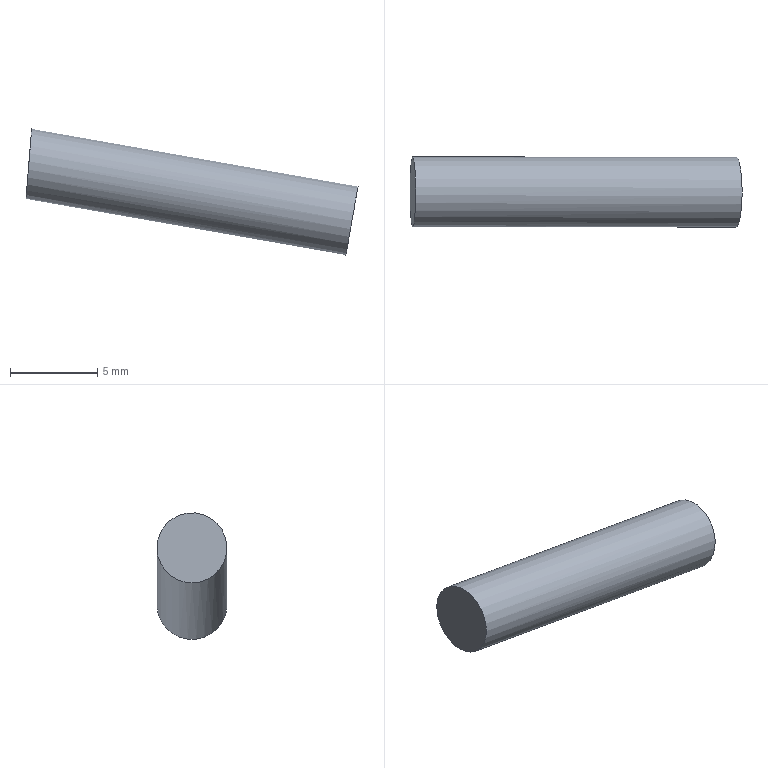Part | NX | features solid 2 | 1 solid | 3 faces | box 18.982 x 4 x 7.23 mm | volume 235.734 mm3 | plane 2 | cylinder 1 | commonest cylinder face diameters 4 x1
STEP:
#1=CARTESIAN_POINT('',(-439.176,690.716,-96.678));
#2=VERTEX_POINT('',#1);
#3=CARTESIAN_POINT('',(-439.176,688.716,-96.678));
#4=DIRECTION('',(-0.9848,0.,0.1736));
#5=DIRECTION('',(0.,1.,0.));
#6=AXIS2_PLACEMENT_3D('',#3,#4,#5);
#7=CIRCLE('',#6,2.);
#8=EDGE_CURVE('',#2,#2,#7,.T.);
#9=ORIENTED_EDGE('',*,*,#8,.T.);
#10=EDGE_LOOP('',(#9));
#11=FACE_BOUND('',#10,.T.);
#12=CARTESIAN_POINT('',(-457.811,688.716,-95.423));
#13=VERTEX_POINT('',#12);
#14=CARTESIAN_POINT('',(-457.65,688.716,-93.42));
#15=DIRECTION('',(-0.9968,0.,0.08003));
#16=DIRECTION('',(-0.08003,0.,-0.9968));
#17=AXIS2_PLACEMENT_3D('',#14,#15,#16);
#18=ELLIPSE('',#17,2.009,2.);
#19=EDGE_CURVE('',#13,#13,#18,.T.);
#20=ORIENTED_EDGE('',*,*,#19,.F.);
#21=EDGE_LOOP('',(#20));
#22=FACE_BOUND('',#21,.T.);
#23=CARTESIAN_POINT('',(-458.872,688.716,-93.205));
#24=DIRECTION('',(0.9848,0.,-0.1736));
#25=DIRECTION('',(0.1736,0.,0.9848));
#26=AXIS2_PLACEMENT_3D('',#23,#24,#25);
#27=CYLINDRICAL_SURFACE('',#26,2.);
#28=ADVANCED_FACE('',(#11,#22),#27,.T.);
#29=ORIENTED_EDGE('',*,*,#8,.F.);
#30=EDGE_LOOP('',(#29));
#31=FACE_BOUND('',#30,.T.);
#32=CARTESIAN_POINT('',(-439.176,688.716,-96.678));
#33=DIRECTION('',(-0.9848,0.,0.1736));
#34=DIRECTION('',(-0.1736,0.,-0.9848));
#35=AXIS2_PLACEMENT_3D('',#32,#33,#34);
#36=PLANE('',#35);
#37=ADVANCED_FACE('',(#31),#36,.F.);
#38=ORIENTED_EDGE('',*,*,#19,.T.);
#39=EDGE_LOOP('',(#38));
#40=FACE_BOUND('',#39,.T.);
#41=CARTESIAN_POINT('',(-448.537,482.597,20.085));
#42=DIRECTION('',(-0.9968,0.,0.08003));
#43=DIRECTION('',(-0.08003,0.,-0.9968));
#44=AXIS2_PLACEMENT_3D('',#41,#42,#43);
#45=PLANE('',#44);
#46=ADVANCED_FACE('',(#40),#45,.T.);
#47=CLOSED_SHELL('',(#28,#37,#46));
#48=MANIFOLD_SOLID_BREP('',#47);
#49=(LENGTH_UNIT()NAMED_UNIT(*)SI_UNIT(.MILLI.,.METRE.));
#50=UNCERTAINTY_MEASURE_WITH_UNIT(LENGTH_MEASURE(0.00001),#49,'','');
#51=(NAMED_UNIT(*)PLANE_ANGLE_UNIT()SI_UNIT($,.RADIAN.));
#52=(NAMED_UNIT(*)SI_UNIT($,.STERADIAN.)SOLID_ANGLE_UNIT());
#53=(GEOMETRIC_REPRESENTATION_CONTEXT(3)GLOBAL_UNCERTAINTY_ASSIGNED_CONTEXT((#50))GLOBAL_UNIT_ASSIGNED_CONTEXT((#49,#51,#52))REPRESENTATION_CONTEXT('',''));
#54=ADVANCED_BREP_SHAPE_REPRESENTATION('',(#48),#53);